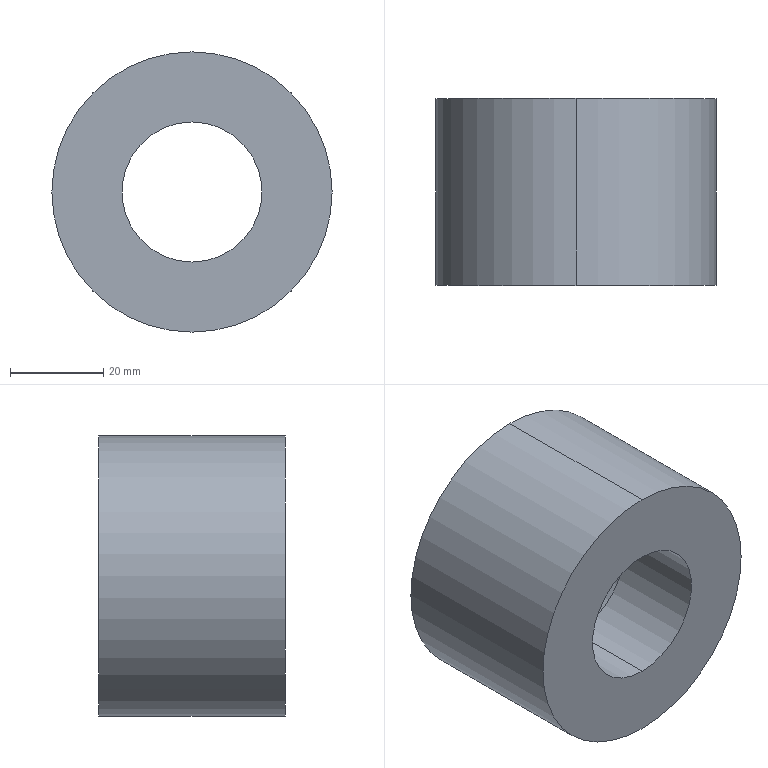Part | SolidWorks | features Revolution 1 | 1 solid | 11 faces | box 60 x 40 x 60 mm | volume 73933 mm3 | cylinder 6 | plane 3 | torus 2 | commonest cylinder face diameters 30 x2 40 x2 60 x2
STEP:
#1=CARTESIAN_POINT('',(0.,-20.,-15.));
#2=VERTEX_POINT('',#1);
#3=CARTESIAN_POINT('',(0.,-20.,15.));
#4=VERTEX_POINT('',#3);
#5=CARTESIAN_POINT('',(0.,-20.,0.));
#6=DIRECTION('',(0.,1.,0.));
#7=DIRECTION('',(0.,0.,1.));
#8=AXIS2_PLACEMENT_3D('',#5,#6,#7);
#9=CIRCLE('',#8,15.);
#10=EDGE_CURVE('',#2,#4,#9,.T.);
#11=ORIENTED_EDGE('',*,*,#10,.F.);
#12=CARTESIAN_POINT('',(0.,0.,-15.));
#13=VERTEX_POINT('',#12);
#14=CARTESIAN_POINT('',(0.,45.568,-15.));
#15=DIRECTION('',(0.,1.,0.));
#16=VECTOR('',#15,1000.);
#17=LINE('',#14,#16);
#18=EDGE_CURVE('',#2,#13,#17,.T.);
#19=ORIENTED_EDGE('',*,*,#18,.T.);
#20=CARTESIAN_POINT('',(0.,0.,15.));
#21=VERTEX_POINT('',#20);
#22=CARTESIAN_POINT('',(0.,0.,0.));
#23=DIRECTION('',(0.,1.,0.));
#24=DIRECTION('',(0.,0.,1.));
#25=AXIS2_PLACEMENT_3D('',#22,#23,#24);
#26=CIRCLE('',#25,15.);
#27=EDGE_CURVE('',#13,#21,#26,.T.);
#28=ORIENTED_EDGE('',*,*,#27,.T.);
#29=CARTESIAN_POINT('',(0.,45.568,15.));
#30=DIRECTION('',(0.,1.,0.));
#31=VECTOR('',#30,1000.);
#32=LINE('',#29,#31);
#33=EDGE_CURVE('',#4,#21,#32,.T.);
#34=ORIENTED_EDGE('',*,*,#33,.F.);
#35=EDGE_LOOP('',(#11,#19,#28,#34));
#36=FACE_OUTER_BOUND('',#35,.T.);
#37=CARTESIAN_POINT('',(0.,45.568,0.));
#38=DIRECTION('',(0.,1.,0.));
#39=DIRECTION('',(0.,0.,1.));
#40=AXIS2_PLACEMENT_3D('',#37,#38,#39);
#41=CYLINDRICAL_SURFACE('',#40,15.);
#42=ADVANCED_FACE('',(#36),#41,.F.);
#43=CARTESIAN_POINT('',(0.,0.,-18.));
#44=VERTEX_POINT('',#43);
#45=CARTESIAN_POINT('',(0.,0.,18.));
#46=VERTEX_POINT('',#45);
#47=CARTESIAN_POINT('',(0.,0.,0.));
#48=DIRECTION('',(0.,1.,0.));
#49=DIRECTION('',(0.,0.,1.));
#50=AXIS2_PLACEMENT_3D('',#47,#48,#49);
#51=CIRCLE('',#50,18.);
#52=EDGE_CURVE('',#44,#46,#51,.T.);
#53=ORIENTED_EDGE('',*,*,#52,.F.);
#54=CARTESIAN_POINT('',(0.,2.,-20.));
#55=VERTEX_POINT('',#54);
#56=CARTESIAN_POINT('',(0.,2.,-18.));
#57=DIRECTION('',(1.,0.,0.));
#58=DIRECTION('',(0.,0.,-1.));
#59=AXIS2_PLACEMENT_3D('',#56,#57,#58);
#60=CIRCLE('',#59,2.);
#61=EDGE_CURVE('',#44,#55,#60,.T.);
#62=ORIENTED_EDGE('',*,*,#61,.T.);
#63=CARTESIAN_POINT('',(0.,2.,20.));
#64=VERTEX_POINT('',#63);
#65=CARTESIAN_POINT('',(0.,2.,0.));
#66=DIRECTION('',(0.,1.,0.));
#67=DIRECTION('',(0.,0.,1.));
#68=AXIS2_PLACEMENT_3D('',#65,#66,#67);
#69=CIRCLE('',#68,20.);
#70=EDGE_CURVE('',#55,#64,#69,.T.);
#71=ORIENTED_EDGE('',*,*,#70,.T.);
#72=CARTESIAN_POINT('',(0.,2.,18.));
#73=DIRECTION('',(-1.,0.,0.));
#74=DIRECTION('',(0.,0.,1.));
#75=AXIS2_PLACEMENT_3D('',#72,#73,#74);
#76=CIRCLE('',#75,2.);
#77=EDGE_CURVE('',#46,#64,#76,.T.);
#78=ORIENTED_EDGE('',*,*,#77,.F.);
#79=EDGE_LOOP('',(#53,#62,#71,#78));
#80=FACE_OUTER_BOUND('',#79,.T.);
#81=CARTESIAN_POINT('',(0.,2.,0.));
#82=DIRECTION('',(0.,1.,0.));
#83=DIRECTION('',(0.,0.,1.));
#84=AXIS2_PLACEMENT_3D('',#81,#82,#83);
#85=TOROIDAL_SURFACE('',#84,18.,2.);
#86=ADVANCED_FACE('',(#80),#85,.F.);
#87=ORIENTED_EDGE('',*,*,#70,.F.);
#88=CARTESIAN_POINT('',(0.,20.,-20.));
#89=VERTEX_POINT('',#88);
#90=CARTESIAN_POINT('',(0.,45.568,-20.));
#91=DIRECTION('',(0.,1.,0.));
#92=VECTOR('',#91,1000.);
#93=LINE('',#90,#92);
#94=EDGE_CURVE('',#55,#89,#93,.T.);
#95=ORIENTED_EDGE('',*,*,#94,.T.);
#96=CARTESIAN_POINT('',(0.,20.,20.));
#97=VERTEX_POINT('',#96);
#98=CARTESIAN_POINT('',(0.,20.,0.));
#99=DIRECTION('',(0.,1.,0.));
#100=DIRECTION('',(0.,0.,1.));
#101=AXIS2_PLACEMENT_3D('',#98,#99,#100);
#102=CIRCLE('',#101,20.);
#103=EDGE_CURVE('',#89,#97,#102,.T.);
#104=ORIENTED_EDGE('',*,*,#103,.T.);
#105=CARTESIAN_POINT('',(0.,45.568,20.));
#106=DIRECTION('',(0.,1.,0.));
#107=VECTOR('',#106,1000.);
#108=LINE('',#105,#107);
#109=EDGE_CURVE('',#64,#97,#108,.T.);
#110=ORIENTED_EDGE('',*,*,#109,.F.);
#111=EDGE_LOOP('',(#87,#95,#104,#110));
#112=FACE_OUTER_BOUND('',#111,.T.);
#113=CARTESIAN_POINT('',(0.,45.568,0.));
#114=DIRECTION('',(0.,1.,0.));
#115=DIRECTION('',(0.,0.,1.));
#116=AXIS2_PLACEMENT_3D('',#113,#114,#115);
#117=CYLINDRICAL_SURFACE('',#116,20.);
#118=ADVANCED_FACE('',(#112),#117,.F.);
#119=CARTESIAN_POINT('',(0.,-20.,30.));
#120=VERTEX_POINT('',#119);
#121=CARTESIAN_POINT('',(0.,-20.,-30.));
#122=VERTEX_POINT('',#121);
#123=CARTESIAN_POINT('',(0.,-20.,0.));
#124=DIRECTION('',(0.,1.,0.));
#125=DIRECTION('',(0.,0.,1.));
#126=AXIS2_PLACEMENT_3D('',#123,#124,#125);
#127=CIRCLE('',#126,30.);
#128=EDGE_CURVE('',#120,#122,#127,.T.);
#129=ORIENTED_EDGE('',*,*,#128,.T.);
#130=CARTESIAN_POINT('',(0.,20.,-30.));
#131=VERTEX_POINT('',#130);
#132=CARTESIAN_POINT('',(0.,45.568,-30.));
#133=DIRECTION('',(0.,1.,0.));
#134=VECTOR('',#133,1000.);
#135=LINE('',#132,#134);
#136=EDGE_CURVE('',#122,#131,#135,.T.);
#137=ORIENTED_EDGE('',*,*,#136,.T.);
#138=CARTESIAN_POINT('',(0.,20.,30.));
#139=VERTEX_POINT('',#138);
#140=CARTESIAN_POINT('',(0.,20.,0.));
#141=DIRECTION('',(0.,1.,0.));
#142=DIRECTION('',(0.,0.,1.));
#143=AXIS2_PLACEMENT_3D('',#140,#141,#142);
#144=CIRCLE('',#143,30.);
#145=EDGE_CURVE('',#139,#131,#144,.T.);
#146=ORIENTED_EDGE('',*,*,#145,.F.);
#147=CARTESIAN_POINT('',(0.,45.568,30.));
#148=DIRECTION('',(0.,1.,0.));
#149=VECTOR('',#148,1000.);
#150=LINE('',#147,#149);
#151=EDGE_CURVE('',#120,#139,#150,.T.);
#152=ORIENTED_EDGE('',*,*,#151,.F.);
#153=EDGE_LOOP('',(#129,#137,#146,#152));
#154=FACE_OUTER_BOUND('',#153,.T.);
#155=CARTESIAN_POINT('',(0.,45.568,0.));
#156=DIRECTION('',(0.,1.,0.));
#157=DIRECTION('',(0.,0.,1.));
#158=AXIS2_PLACEMENT_3D('',#155,#156,#157);
#159=CYLINDRICAL_SURFACE('',#158,30.);
#160=ADVANCED_FACE('',(#154),#159,.T.);
#161=ORIENTED_EDGE('',*,*,#128,.F.);
#162=CARTESIAN_POINT('',(0.,-20.,0.));
#163=DIRECTION('',(0.,1.,0.));
#164=DIRECTION('',(0.,0.,1.));
#165=AXIS2_PLACEMENT_3D('',#162,#163,#164);
#166=CIRCLE('',#165,30.);
#167=EDGE_CURVE('',#122,#120,#166,.T.);
#168=ORIENTED_EDGE('',*,*,#167,.F.);
#169=EDGE_LOOP('',(#161,#168));
#170=FACE_OUTER_BOUND('',#169,.T.);
#171=CARTESIAN_POINT('',(0.,-20.,0.));
#172=DIRECTION('',(0.,1.,0.));
#173=DIRECTION('',(0.,0.,1.));
#174=AXIS2_PLACEMENT_3D('',#171,#172,#173);
#175=CIRCLE('',#174,15.);
#176=EDGE_CURVE('',#4,#2,#175,.T.);
#177=ORIENTED_EDGE('',*,*,#176,.T.);
#178=ORIENTED_EDGE('',*,*,#10,.T.);
#179=EDGE_LOOP('',(#177,#178));
#180=FACE_BOUND('',#179,.T.);
#181=CARTESIAN_POINT('',(30.,-20.,0.));
#182=DIRECTION('',(0.,1.,0.));
#183=DIRECTION('',(0.,0.,1.));
#184=AXIS2_PLACEMENT_3D('',#181,#182,#183);
#185=PLANE('',#184);
#186=ADVANCED_FACE('',(#170,#180),#185,.F.);
#187=ORIENTED_EDGE('',*,*,#136,.F.);
#188=ORIENTED_EDGE('',*,*,#167,.T.);
#189=ORIENTED_EDGE('',*,*,#151,.T.);
#190=CARTESIAN_POINT('',(0.,20.,0.));
#191=DIRECTION('',(0.,1.,0.));
#192=DIRECTION('',(0.,0.,1.));
#193=AXIS2_PLACEMENT_3D('',#190,#191,#192);
#194=CIRCLE('',#193,30.);
#195=EDGE_CURVE('',#131,#139,#194,.T.);
#196=ORIENTED_EDGE('',*,*,#195,.F.);
#197=EDGE_LOOP('',(#187,#188,#189,#196));
#198=FACE_OUTER_BOUND('',#197,.T.);
#199=CARTESIAN_POINT('',(0.,45.568,0.));
#200=DIRECTION('',(0.,1.,0.));
#201=DIRECTION('',(0.,0.,1.));
#202=AXIS2_PLACEMENT_3D('',#199,#200,#201);
#203=CYLINDRICAL_SURFACE('',#202,30.);
#204=ADVANCED_FACE('',(#198),#203,.T.);
#205=CARTESIAN_POINT('',(0.,20.,0.));
#206=DIRECTION('',(0.,1.,0.));
#207=DIRECTION('',(0.,0.,1.));
#208=AXIS2_PLACEMENT_3D('',#205,#206,#207);
#209=CIRCLE('',#208,20.);
#210=EDGE_CURVE('',#97,#89,#209,.T.);
#211=ORIENTED_EDGE('',*,*,#210,.F.);
#212=ORIENTED_EDGE('',*,*,#103,.F.);
#213=EDGE_LOOP('',(#211,#212));
#214=FACE_BOUND('',#213,.T.);
#215=ORIENTED_EDGE('',*,*,#145,.T.);
#216=ORIENTED_EDGE('',*,*,#195,.T.);
#217=EDGE_LOOP('',(#215,#216));
#218=FACE_OUTER_BOUND('',#217,.T.);
#219=CARTESIAN_POINT('',(20.,20.,0.));
#220=DIRECTION('',(0.,-1.,0.));
#221=DIRECTION('',(0.,0.,-1.));
#222=AXIS2_PLACEMENT_3D('',#219,#220,#221);
#223=PLANE('',#222);
#224=ADVANCED_FACE('',(#214,#218),#223,.F.);
#225=ORIENTED_EDGE('',*,*,#94,.F.);
#226=CARTESIAN_POINT('',(0.,2.,0.));
#227=DIRECTION('',(0.,1.,0.));
#228=DIRECTION('',(0.,0.,1.));
#229=AXIS2_PLACEMENT_3D('',#226,#227,#228);
#230=CIRCLE('',#229,20.);
#231=EDGE_CURVE('',#64,#55,#230,.T.);
#232=ORIENTED_EDGE('',*,*,#231,.F.);
#233=ORIENTED_EDGE('',*,*,#109,.T.);
#234=ORIENTED_EDGE('',*,*,#210,.T.);
#235=EDGE_LOOP('',(#225,#232,#233,#234));
#236=FACE_OUTER_BOUND('',#235,.T.);
#237=CARTESIAN_POINT('',(0.,45.568,0.));
#238=DIRECTION('',(0.,1.,0.));
#239=DIRECTION('',(0.,0.,1.));
#240=AXIS2_PLACEMENT_3D('',#237,#238,#239);
#241=CYLINDRICAL_SURFACE('',#240,20.);
#242=ADVANCED_FACE('',(#236),#241,.F.);
#243=ORIENTED_EDGE('',*,*,#61,.F.);
#244=CARTESIAN_POINT('',(0.,0.,0.));
#245=DIRECTION('',(0.,1.,0.));
#246=DIRECTION('',(0.,0.,1.));
#247=AXIS2_PLACEMENT_3D('',#244,#245,#246);
#248=CIRCLE('',#247,18.);
#249=EDGE_CURVE('',#46,#44,#248,.T.);
#250=ORIENTED_EDGE('',*,*,#249,.F.);
#251=ORIENTED_EDGE('',*,*,#77,.T.);
#252=ORIENTED_EDGE('',*,*,#231,.T.);
#253=EDGE_LOOP('',(#243,#250,#251,#252));
#254=FACE_OUTER_BOUND('',#253,.T.);
#255=CARTESIAN_POINT('',(0.,2.,0.));
#256=DIRECTION('',(0.,1.,0.));
#257=DIRECTION('',(0.,0.,1.));
#258=AXIS2_PLACEMENT_3D('',#255,#256,#257);
#259=TOROIDAL_SURFACE('',#258,18.,2.);
#260=ADVANCED_FACE('',(#254),#259,.F.);
#261=CARTESIAN_POINT('',(0.,0.,0.));
#262=DIRECTION('',(0.,1.,0.));
#263=DIRECTION('',(0.,0.,1.));
#264=AXIS2_PLACEMENT_3D('',#261,#262,#263);
#265=CIRCLE('',#264,15.);
#266=EDGE_CURVE('',#21,#13,#265,.T.);
#267=ORIENTED_EDGE('',*,*,#266,.F.);
#268=ORIENTED_EDGE('',*,*,#27,.F.);
#269=EDGE_LOOP('',(#267,#268));
#270=FACE_BOUND('',#269,.T.);
#271=ORIENTED_EDGE('',*,*,#249,.T.);
#272=ORIENTED_EDGE('',*,*,#52,.T.);
#273=EDGE_LOOP('',(#271,#272));
#274=FACE_OUTER_BOUND('',#273,.T.);
#275=CARTESIAN_POINT('',(15.,0.,0.));
#276=DIRECTION('',(0.,-1.,0.));
#277=DIRECTION('',(0.,0.,-1.));
#278=AXIS2_PLACEMENT_3D('',#275,#276,#277);
#279=PLANE('',#278);
#280=ADVANCED_FACE('',(#270,#274),#279,.F.);
#281=ORIENTED_EDGE('',*,*,#18,.F.);
#282=ORIENTED_EDGE('',*,*,#176,.F.);
#283=ORIENTED_EDGE('',*,*,#33,.T.);
#284=ORIENTED_EDGE('',*,*,#266,.T.);
#285=EDGE_LOOP('',(#281,#282,#283,#284));
#286=FACE_OUTER_BOUND('',#285,.T.);
#287=CARTESIAN_POINT('',(0.,45.568,0.));
#288=DIRECTION('',(0.,1.,0.));
#289=DIRECTION('',(0.,0.,1.));
#290=AXIS2_PLACEMENT_3D('',#287,#288,#289);
#291=CYLINDRICAL_SURFACE('',#290,15.);
#292=ADVANCED_FACE('',(#286),#291,.F.);
#293=CLOSED_SHELL('',(#42,#86,#118,#160,#186,#204,#224,#242,#260,#280,#292));
#294=MANIFOLD_SOLID_BREP('',#293);
#295=CARTESIAN_POINT('',(0.,0.,0.));
#296=DIRECTION('',(0.,0.,1.));
#297=DIRECTION('',(1.,0.,0.));
#298=AXIS2_PLACEMENT_3D('',#295,#296,#297);
#299=(LENGTH_UNIT()NAMED_UNIT(*)SI_UNIT(.MILLI.,.METRE.));
#300=UNCERTAINTY_MEASURE_WITH_UNIT(LENGTH_MEASURE(0.00001),#299,'','');
#301=(NAMED_UNIT(*)PLANE_ANGLE_UNIT()SI_UNIT($,.RADIAN.));
#302=(NAMED_UNIT(*)SI_UNIT($,.STERADIAN.)SOLID_ANGLE_UNIT());
#303=(GEOMETRIC_REPRESENTATION_CONTEXT(3)GLOBAL_UNCERTAINTY_ASSIGNED_CONTEXT((#300))GLOBAL_UNIT_ASSIGNED_CONTEXT((#299,#301,#302))REPRESENTATION_CONTEXT('',''));
#304=ADVANCED_BREP_SHAPE_REPRESENTATION('',(#294,#298),#303);